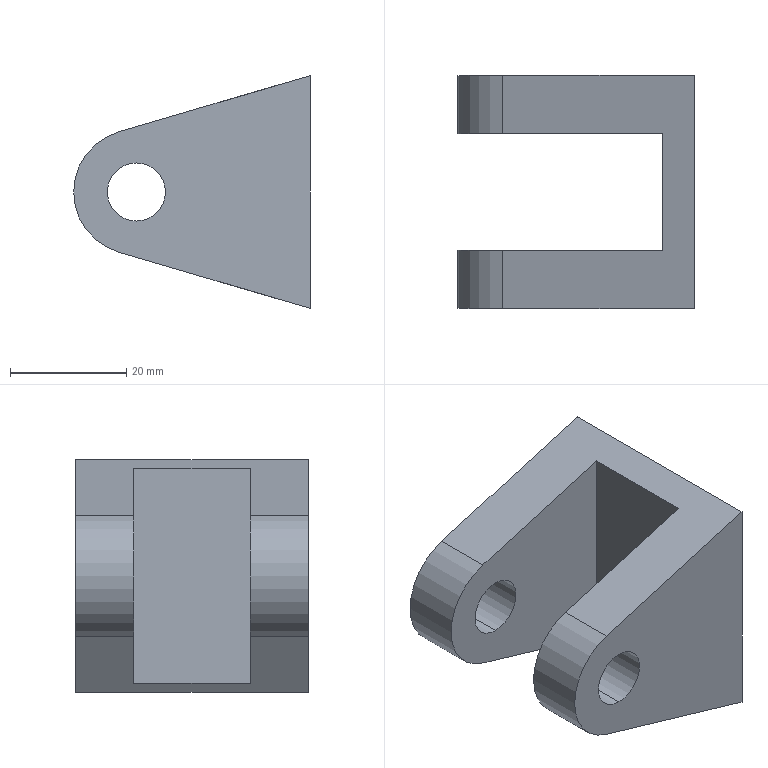Part | SolidWorks | features ICE 2, Extrusion 1 | 1 solid | 14 faces | box 40.645 x 40 x 40 mm | volume 24880 mm3 | plane 8 | cylinder 6 | commonest cylinder face diameters 10 x4 21.526 x2
STEP:
#1=CARTESIAN_POINT('',(-29.882,40.,25.));
#2=VERTEX_POINT('',#1);
#3=CARTESIAN_POINT('',(-29.882,40.,15.));
#4=VERTEX_POINT('',#3);
#5=CARTESIAN_POINT('',(-29.882,40.,20.));
#6=DIRECTION('',(0.,-1.,0.));
#7=DIRECTION('',(0.,0.,-1.));
#8=AXIS2_PLACEMENT_3D('',#5,#6,#7);
#9=CIRCLE('',#8,5.);
#10=EDGE_CURVE('',#2,#4,#9,.T.);
#11=ORIENTED_EDGE('',*,*,#10,.F.);
#12=CARTESIAN_POINT('',(-29.882,30.,25.));
#13=VERTEX_POINT('',#12);
#14=CARTESIAN_POINT('',(-29.882,80.,25.));
#15=DIRECTION('',(0.,-1.,0.));
#16=VECTOR('',#15,1000.);
#17=LINE('',#14,#16);
#18=EDGE_CURVE('',#2,#13,#17,.T.);
#19=ORIENTED_EDGE('',*,*,#18,.T.);
#20=CARTESIAN_POINT('',(-29.882,30.,15.));
#21=VERTEX_POINT('',#20);
#22=CARTESIAN_POINT('',(-29.882,30.,20.));
#23=DIRECTION('',(0.,-1.,0.));
#24=DIRECTION('',(0.,0.,-1.));
#25=AXIS2_PLACEMENT_3D('',#22,#23,#24);
#26=CIRCLE('',#25,5.);
#27=EDGE_CURVE('',#13,#21,#26,.T.);
#28=ORIENTED_EDGE('',*,*,#27,.T.);
#29=CARTESIAN_POINT('',(-29.882,80.,15.));
#30=DIRECTION('',(0.,-1.,0.));
#31=VECTOR('',#30,1000.);
#32=LINE('',#29,#31);
#33=EDGE_CURVE('',#4,#21,#32,.T.);
#34=ORIENTED_EDGE('',*,*,#33,.F.);
#35=EDGE_LOOP('',(#11,#19,#28,#34));
#36=FACE_OUTER_BOUND('',#35,.T.);
#37=CARTESIAN_POINT('',(-29.882,80.,20.));
#38=DIRECTION('',(0.,-1.,0.));
#39=DIRECTION('',(0.,0.,-1.));
#40=AXIS2_PLACEMENT_3D('',#37,#38,#39);
#41=CYLINDRICAL_SURFACE('',#40,5.);
#42=ADVANCED_FACE('',(#36),#41,.F.);
#43=CARTESIAN_POINT('',(-29.882,10.,25.));
#44=VERTEX_POINT('',#43);
#45=CARTESIAN_POINT('',(-29.882,10.,15.));
#46=VERTEX_POINT('',#45);
#47=CARTESIAN_POINT('',(-29.882,10.,20.));
#48=DIRECTION('',(0.,-1.,0.));
#49=DIRECTION('',(0.,0.,-1.));
#50=AXIS2_PLACEMENT_3D('',#47,#48,#49);
#51=CIRCLE('',#50,5.);
#52=EDGE_CURVE('',#44,#46,#51,.T.);
#53=ORIENTED_EDGE('',*,*,#52,.F.);
#54=CARTESIAN_POINT('',(-29.882,0.,25.));
#55=VERTEX_POINT('',#54);
#56=CARTESIAN_POINT('',(-29.882,80.,25.));
#57=DIRECTION('',(0.,-1.,0.));
#58=VECTOR('',#57,1000.);
#59=LINE('',#56,#58);
#60=EDGE_CURVE('',#44,#55,#59,.T.);
#61=ORIENTED_EDGE('',*,*,#60,.T.);
#62=CARTESIAN_POINT('',(-29.882,0.,15.));
#63=VERTEX_POINT('',#62);
#64=CARTESIAN_POINT('',(-29.882,0.,20.));
#65=DIRECTION('',(0.,-1.,0.));
#66=DIRECTION('',(0.,0.,-1.));
#67=AXIS2_PLACEMENT_3D('',#64,#65,#66);
#68=CIRCLE('',#67,5.);
#69=EDGE_CURVE('',#55,#63,#68,.T.);
#70=ORIENTED_EDGE('',*,*,#69,.T.);
#71=CARTESIAN_POINT('',(-29.882,80.,15.));
#72=DIRECTION('',(0.,-1.,0.));
#73=VECTOR('',#72,1000.);
#74=LINE('',#71,#73);
#75=EDGE_CURVE('',#46,#63,#74,.T.);
#76=ORIENTED_EDGE('',*,*,#75,.F.);
#77=EDGE_LOOP('',(#53,#61,#70,#76));
#78=FACE_OUTER_BOUND('',#77,.T.);
#79=CARTESIAN_POINT('',(-29.882,80.,20.));
#80=DIRECTION('',(0.,-1.,0.));
#81=DIRECTION('',(0.,0.,-1.));
#82=AXIS2_PLACEMENT_3D('',#79,#80,#81);
#83=CYLINDRICAL_SURFACE('',#82,5.);
#84=ADVANCED_FACE('',(#78),#83,.F.);
#85=CARTESIAN_POINT('',(-32.917,30.,9.673));
#86=VERTEX_POINT('',#85);
#87=CARTESIAN_POINT('',(-5.382,30.,1.581));
#88=VERTEX_POINT('',#87);
#89=CARTESIAN_POINT('',(-32.917,30.,9.673));
#90=DIRECTION('',(0.9594,0.,-0.282));
#91=VECTOR('',#90,1000.);
#92=LINE('',#89,#91);
#93=EDGE_CURVE('',#86,#88,#92,.T.);
#94=ORIENTED_EDGE('',*,*,#93,.F.);
#95=CARTESIAN_POINT('',(-32.917,40.,9.673));
#96=VERTEX_POINT('',#95);
#97=CARTESIAN_POINT('',(-32.917,40.,9.673));
#98=DIRECTION('',(0.,-1.,0.));
#99=VECTOR('',#98,1000.);
#100=LINE('',#97,#99);
#101=EDGE_CURVE('',#96,#86,#100,.T.);
#102=ORIENTED_EDGE('',*,*,#101,.F.);
#103=CARTESIAN_POINT('',(0.,40.,0.));
#104=VERTEX_POINT('',#103);
#105=CARTESIAN_POINT('',(0.,40.,0.));
#106=DIRECTION('',(-0.9594,0.,0.282));
#107=VECTOR('',#106,1000.);
#108=LINE('',#105,#107);
#109=EDGE_CURVE('',#104,#96,#108,.T.);
#110=ORIENTED_EDGE('',*,*,#109,.F.);
#111=CARTESIAN_POINT('',(0.,0.,0.));
#112=VERTEX_POINT('',#111);
#113=CARTESIAN_POINT('',(0.,40.,0.));
#114=DIRECTION('',(0.,-1.,0.));
#115=VECTOR('',#114,1000.);
#116=LINE('',#113,#115);
#117=EDGE_CURVE('',#104,#112,#116,.T.);
#118=ORIENTED_EDGE('',*,*,#117,.T.);
#119=CARTESIAN_POINT('',(-32.917,0.,9.673));
#120=VERTEX_POINT('',#119);
#121=CARTESIAN_POINT('',(0.,0.,0.));
#122=DIRECTION('',(-0.9594,0.,0.282));
#123=VECTOR('',#122,1000.);
#124=LINE('',#121,#123);
#125=EDGE_CURVE('',#112,#120,#124,.T.);
#126=ORIENTED_EDGE('',*,*,#125,.T.);
#127=CARTESIAN_POINT('',(-32.917,10.,9.673));
#128=VERTEX_POINT('',#127);
#129=CARTESIAN_POINT('',(-32.917,40.,9.673));
#130=DIRECTION('',(0.,-1.,0.));
#131=VECTOR('',#130,1000.);
#132=LINE('',#129,#131);
#133=EDGE_CURVE('',#128,#120,#132,.T.);
#134=ORIENTED_EDGE('',*,*,#133,.F.);
#135=CARTESIAN_POINT('',(-5.382,10.,1.581));
#136=VERTEX_POINT('',#135);
#137=CARTESIAN_POINT('',(-32.917,10.,9.673));
#138=DIRECTION('',(0.9594,0.,-0.282));
#139=VECTOR('',#138,1000.);
#140=LINE('',#137,#139);
#141=EDGE_CURVE('',#128,#136,#140,.T.);
#142=ORIENTED_EDGE('',*,*,#141,.T.);
#143=CARTESIAN_POINT('',(-5.382,30.,1.581));
#144=DIRECTION('',(0.,-1.,0.));
#145=VECTOR('',#144,1000.);
#146=LINE('',#143,#145);
#147=EDGE_CURVE('',#88,#136,#146,.T.);
#148=ORIENTED_EDGE('',*,*,#147,.F.);
#149=EDGE_LOOP('',(#94,#102,#110,#118,#126,#134,#142,#148));
#150=FACE_OUTER_BOUND('',#149,.T.);
#151=CARTESIAN_POINT('',(0.,40.,0.));
#152=DIRECTION('',(0.282,0.,0.9594));
#153=DIRECTION('',(0.9594,0.,-0.282));
#154=AXIS2_PLACEMENT_3D('',#151,#152,#153);
#155=PLANE('',#154);
#156=ADVANCED_FACE('',(#150),#155,.F.);
#157=CARTESIAN_POINT('',(-32.917,30.,30.327));
#158=VERTEX_POINT('',#157);
#159=CARTESIAN_POINT('',(-29.882,30.,20.));
#160=DIRECTION('',(0.,-1.,0.));
#161=DIRECTION('',(0.,0.,-1.));
#162=AXIS2_PLACEMENT_3D('',#159,#160,#161);
#163=CIRCLE('',#162,10.763);
#164=EDGE_CURVE('',#158,#86,#163,.T.);
#165=ORIENTED_EDGE('',*,*,#164,.F.);
#166=CARTESIAN_POINT('',(-32.917,40.,30.327));
#167=VERTEX_POINT('',#166);
#168=CARTESIAN_POINT('',(-32.917,40.,30.327));
#169=DIRECTION('',(0.,-1.,0.));
#170=VECTOR('',#169,1000.);
#171=LINE('',#168,#170);
#172=EDGE_CURVE('',#167,#158,#171,.T.);
#173=ORIENTED_EDGE('',*,*,#172,.F.);
#174=CARTESIAN_POINT('',(-29.882,40.,20.));
#175=DIRECTION('',(0.,1.,0.));
#176=DIRECTION('',(0.,0.,-1.));
#177=AXIS2_PLACEMENT_3D('',#174,#175,#176);
#178=CIRCLE('',#177,10.763);
#179=EDGE_CURVE('',#96,#167,#178,.T.);
#180=ORIENTED_EDGE('',*,*,#179,.F.);
#181=ORIENTED_EDGE('',*,*,#101,.T.);
#182=EDGE_LOOP('',(#165,#173,#180,#181));
#183=FACE_OUTER_BOUND('',#182,.T.);
#184=CARTESIAN_POINT('',(-29.882,40.,20.));
#185=DIRECTION('',(0.,-1.,0.));
#186=DIRECTION('',(0.,0.,-1.));
#187=AXIS2_PLACEMENT_3D('',#184,#185,#186);
#188=CYLINDRICAL_SURFACE('',#187,10.763);
#189=ADVANCED_FACE('',(#183),#188,.T.);
#190=CARTESIAN_POINT('',(-5.382,30.,38.419));
#191=VERTEX_POINT('',#190);
#192=CARTESIAN_POINT('',(-5.382,30.,38.419));
#193=DIRECTION('',(-0.9594,0.,-0.282));
#194=VECTOR('',#193,1000.);
#195=LINE('',#192,#194);
#196=EDGE_CURVE('',#191,#158,#195,.T.);
#197=ORIENTED_EDGE('',*,*,#196,.F.);
#198=CARTESIAN_POINT('',(-5.382,10.,38.419));
#199=VERTEX_POINT('',#198);
#200=CARTESIAN_POINT('',(-5.382,30.,38.419));
#201=DIRECTION('',(0.,-1.,0.));
#202=VECTOR('',#201,1000.);
#203=LINE('',#200,#202);
#204=EDGE_CURVE('',#191,#199,#203,.T.);
#205=ORIENTED_EDGE('',*,*,#204,.T.);
#206=CARTESIAN_POINT('',(-32.917,10.,30.327));
#207=VERTEX_POINT('',#206);
#208=CARTESIAN_POINT('',(-5.382,10.,38.419));
#209=DIRECTION('',(-0.9594,0.,-0.282));
#210=VECTOR('',#209,1000.);
#211=LINE('',#208,#210);
#212=EDGE_CURVE('',#199,#207,#211,.T.);
#213=ORIENTED_EDGE('',*,*,#212,.T.);
#214=CARTESIAN_POINT('',(-32.917,0.,30.327));
#215=VERTEX_POINT('',#214);
#216=CARTESIAN_POINT('',(-32.917,40.,30.327));
#217=DIRECTION('',(0.,-1.,0.));
#218=VECTOR('',#217,1000.);
#219=LINE('',#216,#218);
#220=EDGE_CURVE('',#207,#215,#219,.T.);
#221=ORIENTED_EDGE('',*,*,#220,.T.);
#222=CARTESIAN_POINT('',(0.,0.,40.));
#223=VERTEX_POINT('',#222);
#224=CARTESIAN_POINT('',(0.,0.,40.));
#225=DIRECTION('',(0.9594,0.,0.282));
#226=VECTOR('',#225,1000.);
#227=LINE('',#224,#226);
#228=EDGE_CURVE('',#215,#223,#227,.T.);
#229=ORIENTED_EDGE('',*,*,#228,.T.);
#230=CARTESIAN_POINT('',(0.,40.,40.));
#231=VERTEX_POINT('',#230);
#232=CARTESIAN_POINT('',(0.,40.,40.));
#233=DIRECTION('',(0.,-1.,0.));
#234=VECTOR('',#233,1000.);
#235=LINE('',#232,#234);
#236=EDGE_CURVE('',#231,#223,#235,.T.);
#237=ORIENTED_EDGE('',*,*,#236,.F.);
#238=CARTESIAN_POINT('',(0.,40.,40.));
#239=DIRECTION('',(0.9594,0.,0.282));
#240=VECTOR('',#239,1000.);
#241=LINE('',#238,#240);
#242=EDGE_CURVE('',#167,#231,#241,.T.);
#243=ORIENTED_EDGE('',*,*,#242,.F.);
#244=ORIENTED_EDGE('',*,*,#172,.T.);
#245=EDGE_LOOP('',(#197,#205,#213,#221,#229,#237,#243,#244));
#246=FACE_OUTER_BOUND('',#245,.T.);
#247=CARTESIAN_POINT('',(0.,40.,40.));
#248=DIRECTION('',(0.282,0.,-0.9594));
#249=DIRECTION('',(-0.9594,0.,-0.282));
#250=AXIS2_PLACEMENT_3D('',#247,#248,#249);
#251=PLANE('',#250);
#252=ADVANCED_FACE('',(#246),#251,.F.);
#253=ORIENTED_EDGE('',*,*,#220,.F.);
#254=CARTESIAN_POINT('',(-29.882,10.,20.));
#255=DIRECTION('',(0.,-1.,0.));
#256=DIRECTION('',(0.,0.,-1.));
#257=AXIS2_PLACEMENT_3D('',#254,#255,#256);
#258=CIRCLE('',#257,10.763);
#259=EDGE_CURVE('',#207,#128,#258,.T.);
#260=ORIENTED_EDGE('',*,*,#259,.T.);
#261=ORIENTED_EDGE('',*,*,#133,.T.);
#262=CARTESIAN_POINT('',(-29.882,0.,20.));
#263=DIRECTION('',(0.,1.,0.));
#264=DIRECTION('',(0.,0.,-1.));
#265=AXIS2_PLACEMENT_3D('',#262,#263,#264);
#266=CIRCLE('',#265,10.763);
#267=EDGE_CURVE('',#120,#215,#266,.T.);
#268=ORIENTED_EDGE('',*,*,#267,.T.);
#269=EDGE_LOOP('',(#253,#260,#261,#268));
#270=FACE_OUTER_BOUND('',#269,.T.);
#271=CARTESIAN_POINT('',(-29.882,40.,20.));
#272=DIRECTION('',(0.,-1.,0.));
#273=DIRECTION('',(0.,0.,-1.));
#274=AXIS2_PLACEMENT_3D('',#271,#272,#273);
#275=CYLINDRICAL_SURFACE('',#274,10.763);
#276=ADVANCED_FACE('',(#270),#275,.T.);
#277=CARTESIAN_POINT('',(0.,0.,0.));
#278=DIRECTION('',(0.,0.,-1.));
#279=VECTOR('',#278,1000.);
#280=LINE('',#277,#279);
#281=EDGE_CURVE('',#223,#112,#280,.T.);
#282=ORIENTED_EDGE('',*,*,#281,.T.);
#283=ORIENTED_EDGE('',*,*,#117,.F.);
#284=CARTESIAN_POINT('',(0.,40.,0.));
#285=DIRECTION('',(0.,0.,-1.));
#286=VECTOR('',#285,1000.);
#287=LINE('',#284,#286);
#288=EDGE_CURVE('',#231,#104,#287,.T.);
#289=ORIENTED_EDGE('',*,*,#288,.F.);
#290=ORIENTED_EDGE('',*,*,#236,.T.);
#291=EDGE_LOOP('',(#282,#283,#289,#290));
#292=FACE_OUTER_BOUND('',#291,.T.);
#293=CARTESIAN_POINT('',(0.,40.,0.));
#294=DIRECTION('',(-1.,0.,0.));
#295=DIRECTION('',(0.,0.,1.));
#296=AXIS2_PLACEMENT_3D('',#293,#294,#295);
#297=PLANE('',#296);
#298=ADVANCED_FACE('',(#292),#297,.F.);
#299=CARTESIAN_POINT('',(-29.882,40.,20.));
#300=DIRECTION('',(0.,-1.,0.));
#301=DIRECTION('',(0.,0.,-1.));
#302=AXIS2_PLACEMENT_3D('',#299,#300,#301);
#303=CIRCLE('',#302,5.);
#304=EDGE_CURVE('',#4,#2,#303,.T.);
#305=ORIENTED_EDGE('',*,*,#304,.T.);
#306=ORIENTED_EDGE('',*,*,#10,.T.);
#307=EDGE_LOOP('',(#305,#306));
#308=FACE_BOUND('',#307,.T.);
#309=ORIENTED_EDGE('',*,*,#109,.T.);
#310=ORIENTED_EDGE('',*,*,#179,.T.);
#311=ORIENTED_EDGE('',*,*,#242,.T.);
#312=ORIENTED_EDGE('',*,*,#288,.T.);
#313=EDGE_LOOP('',(#309,#310,#311,#312));
#314=FACE_OUTER_BOUND('',#313,.T.);
#315=CARTESIAN_POINT('',(-29.882,40.,20.));
#316=DIRECTION('',(0.,-1.,0.));
#317=DIRECTION('',(0.,0.,-1.));
#318=AXIS2_PLACEMENT_3D('',#315,#316,#317);
#319=PLANE('',#318);
#320=ADVANCED_FACE('',(#308,#314),#319,.F.);
#321=CARTESIAN_POINT('',(-29.882,0.,20.));
#322=DIRECTION('',(0.,-1.,0.));
#323=DIRECTION('',(0.,0.,-1.));
#324=AXIS2_PLACEMENT_3D('',#321,#322,#323);
#325=CIRCLE('',#324,5.);
#326=EDGE_CURVE('',#63,#55,#325,.T.);
#327=ORIENTED_EDGE('',*,*,#326,.F.);
#328=ORIENTED_EDGE('',*,*,#69,.F.);
#329=EDGE_LOOP('',(#327,#328));
#330=FACE_BOUND('',#329,.T.);
#331=ORIENTED_EDGE('',*,*,#125,.F.);
#332=ORIENTED_EDGE('',*,*,#281,.F.);
#333=ORIENTED_EDGE('',*,*,#228,.F.);
#334=ORIENTED_EDGE('',*,*,#267,.F.);
#335=EDGE_LOOP('',(#331,#332,#333,#334));
#336=FACE_OUTER_BOUND('',#335,.T.);
#337=CARTESIAN_POINT('',(-29.882,0.,20.));
#338=DIRECTION('',(0.,-1.,0.));
#339=DIRECTION('',(0.,0.,-1.));
#340=AXIS2_PLACEMENT_3D('',#337,#338,#339);
#341=PLANE('',#340);
#342=ADVANCED_FACE('',(#330,#336),#341,.T.);
#343=CARTESIAN_POINT('',(-5.382,10.,1.581));
#344=DIRECTION('',(0.,0.,1.));
#345=VECTOR('',#344,1000.);
#346=LINE('',#343,#345);
#347=EDGE_CURVE('',#136,#199,#346,.T.);
#348=ORIENTED_EDGE('',*,*,#347,.T.);
#349=ORIENTED_EDGE('',*,*,#204,.F.);
#350=CARTESIAN_POINT('',(-5.382,30.,1.581));
#351=DIRECTION('',(0.,0.,1.));
#352=VECTOR('',#351,1000.);
#353=LINE('',#350,#352);
#354=EDGE_CURVE('',#88,#191,#353,.T.);
#355=ORIENTED_EDGE('',*,*,#354,.F.);
#356=ORIENTED_EDGE('',*,*,#147,.T.);
#357=EDGE_LOOP('',(#348,#349,#355,#356));
#358=FACE_OUTER_BOUND('',#357,.T.);
#359=CARTESIAN_POINT('',(-5.382,30.,1.581));
#360=DIRECTION('',(1.,0.,0.));
#361=DIRECTION('',(0.,0.,-1.));
#362=AXIS2_PLACEMENT_3D('',#359,#360,#361);
#363=PLANE('',#362);
#364=ADVANCED_FACE('',(#358),#363,.F.);
#365=CARTESIAN_POINT('',(-29.882,30.,20.));
#366=DIRECTION('',(0.,-1.,0.));
#367=DIRECTION('',(0.,0.,-1.));
#368=AXIS2_PLACEMENT_3D('',#365,#366,#367);
#369=CIRCLE('',#368,5.);
#370=EDGE_CURVE('',#21,#13,#369,.T.);
#371=ORIENTED_EDGE('',*,*,#370,.F.);
#372=ORIENTED_EDGE('',*,*,#27,.F.);
#373=EDGE_LOOP('',(#371,#372));
#374=FACE_BOUND('',#373,.T.);
#375=ORIENTED_EDGE('',*,*,#93,.T.);
#376=ORIENTED_EDGE('',*,*,#354,.T.);
#377=ORIENTED_EDGE('',*,*,#196,.T.);
#378=ORIENTED_EDGE('',*,*,#164,.T.);
#379=EDGE_LOOP('',(#375,#376,#377,#378));
#380=FACE_OUTER_BOUND('',#379,.T.);
#381=CARTESIAN_POINT('',(-29.882,30.,20.));
#382=DIRECTION('',(0.,-1.,0.));
#383=DIRECTION('',(0.,0.,-1.));
#384=AXIS2_PLACEMENT_3D('',#381,#382,#383);
#385=PLANE('',#384);
#386=ADVANCED_FACE('',(#374,#380),#385,.T.);
#387=CARTESIAN_POINT('',(-29.882,10.,20.));
#388=DIRECTION('',(0.,-1.,0.));
#389=DIRECTION('',(0.,0.,-1.));
#390=AXIS2_PLACEMENT_3D('',#387,#388,#389);
#391=CIRCLE('',#390,5.);
#392=EDGE_CURVE('',#46,#44,#391,.T.);
#393=ORIENTED_EDGE('',*,*,#392,.T.);
#394=ORIENTED_EDGE('',*,*,#52,.T.);
#395=EDGE_LOOP('',(#393,#394));
#396=FACE_BOUND('',#395,.T.);
#397=ORIENTED_EDGE('',*,*,#141,.F.);
#398=ORIENTED_EDGE('',*,*,#259,.F.);
#399=ORIENTED_EDGE('',*,*,#212,.F.);
#400=ORIENTED_EDGE('',*,*,#347,.F.);
#401=EDGE_LOOP('',(#397,#398,#399,#400));
#402=FACE_OUTER_BOUND('',#401,.T.);
#403=CARTESIAN_POINT('',(-29.882,10.,20.));
#404=DIRECTION('',(0.,-1.,0.));
#405=DIRECTION('',(0.,0.,-1.));
#406=AXIS2_PLACEMENT_3D('',#403,#404,#405);
#407=PLANE('',#406);
#408=ADVANCED_FACE('',(#396,#402),#407,.F.);
#409=ORIENTED_EDGE('',*,*,#60,.F.);
#410=ORIENTED_EDGE('',*,*,#392,.F.);
#411=ORIENTED_EDGE('',*,*,#75,.T.);
#412=ORIENTED_EDGE('',*,*,#326,.T.);
#413=EDGE_LOOP('',(#409,#410,#411,#412));
#414=FACE_OUTER_BOUND('',#413,.T.);
#415=CARTESIAN_POINT('',(-29.882,80.,20.));
#416=DIRECTION('',(0.,-1.,0.));
#417=DIRECTION('',(0.,0.,-1.));
#418=AXIS2_PLACEMENT_3D('',#415,#416,#417);
#419=CYLINDRICAL_SURFACE('',#418,5.);
#420=ADVANCED_FACE('',(#414),#419,.F.);
#421=ORIENTED_EDGE('',*,*,#18,.F.);
#422=ORIENTED_EDGE('',*,*,#304,.F.);
#423=ORIENTED_EDGE('',*,*,#33,.T.);
#424=ORIENTED_EDGE('',*,*,#370,.T.);
#425=EDGE_LOOP('',(#421,#422,#423,#424));
#426=FACE_OUTER_BOUND('',#425,.T.);
#427=CARTESIAN_POINT('',(-29.882,80.,20.));
#428=DIRECTION('',(0.,-1.,0.));
#429=DIRECTION('',(0.,0.,-1.));
#430=AXIS2_PLACEMENT_3D('',#427,#428,#429);
#431=CYLINDRICAL_SURFACE('',#430,5.);
#432=ADVANCED_FACE('',(#426),#431,.F.);
#433=CLOSED_SHELL('',(#42,#84,#156,#189,#252,#276,#298,#320,#342,#364,#386,#408,#420,#432));
#434=MANIFOLD_SOLID_BREP('',#433);
#435=CARTESIAN_POINT('',(0.,0.,0.));
#436=DIRECTION('',(0.,0.,1.));
#437=DIRECTION('',(1.,0.,0.));
#438=AXIS2_PLACEMENT_3D('',#435,#436,#437);
#439=(LENGTH_UNIT()NAMED_UNIT(*)SI_UNIT(.MILLI.,.METRE.));
#440=UNCERTAINTY_MEASURE_WITH_UNIT(LENGTH_MEASURE(0.00001),#439,'','');
#441=(NAMED_UNIT(*)PLANE_ANGLE_UNIT()SI_UNIT($,.RADIAN.));
#442=(NAMED_UNIT(*)SI_UNIT($,.STERADIAN.)SOLID_ANGLE_UNIT());
#443=(GEOMETRIC_REPRESENTATION_CONTEXT(3)GLOBAL_UNCERTAINTY_ASSIGNED_CONTEXT((#440))GLOBAL_UNIT_ASSIGNED_CONTEXT((#439,#441,#442))REPRESENTATION_CONTEXT('',''));
#444=ADVANCED_BREP_SHAPE_REPRESENTATION('',(#434,#438),#443);